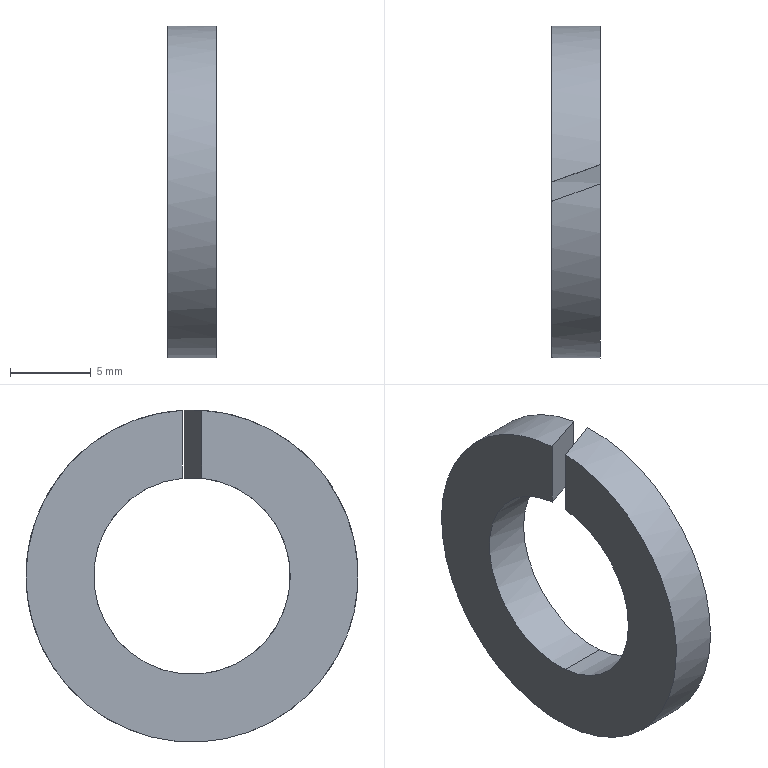Part | STEP file | KS B 1324 - No. 2 - 12 | 1 solid | 8 faces | box 3 x 20.6 x 20.6 mm | volume 633.995 mm3 | cylinder 4 | plane 4 | commonest cylinder face diameters 12.2 x2 20.6 x2
STEP:
#1=CARTESIAN_POINT('',(0.,0.,0.));
#2=DIRECTION('',(0.,0.,1.));
#3=DIRECTION('',(1.,0.,0.));
#4=AXIS2_PLACEMENT_3D('',#1,#2,#3);
#5=CARTESIAN_POINT('',(3.,1.692,5.861));
#6=VERTEX_POINT('',#5);
#7=CARTESIAN_POINT('',(0.,0.6,6.07));
#8=VERTEX_POINT('',#7);
#9=CARTESIAN_POINT('',(3.,1.692,5.861));
#10=CARTESIAN_POINT('',(2.019,1.335,5.964));
#11=CARTESIAN_POINT('',(1.016,0.9699,6.034));
#12=CARTESIAN_POINT('',(0.,0.6,6.07));
#13=(BOUNDED_CURVE()B_SPLINE_CURVE(3,(#9,#10,#11,#12),.UNSPECIFIED.,.F.,.F.)B_SPLINE_CURVE_WITH_KNOTS((4,4),(4.431,4.614),.PIECEWISE_BEZIER_KNOTS.)CURVE()GEOMETRIC_REPRESENTATION_ITEM()RATIONAL_B_SPLINE_CURVE((1.,0.9972,0.9972,1.))REPRESENTATION_ITEM(''));
#14=CARTESIAN_POINT('',(0.,0.,0.));
#15=DIRECTION('',(1.,0.,0.));
#16=DIRECTION('',(0.,-0.0895,-0.996));
#17=AXIS2_PLACEMENT_3D('',#14,#15,#16);
#18=CYLINDRICAL_SURFACE('',#17,6.1);
#19=CARTESIAN_POINT('',(2.95,3.));
#20=CARTESIAN_POINT('',(2.953,2.956));
#21=CARTESIAN_POINT('',(2.958,2.866));
#22=CARTESIAN_POINT('',(2.967,2.733));
#23=CARTESIAN_POINT('',(2.975,2.598));
#24=CARTESIAN_POINT('',(2.983,2.464));
#25=CARTESIAN_POINT('',(2.992,2.329));
#26=CARTESIAN_POINT('',(3.,2.193));
#27=CARTESIAN_POINT('',(3.008,2.058));
#28=CARTESIAN_POINT('',(3.017,1.922));
#29=CARTESIAN_POINT('',(3.025,1.786));
#30=CARTESIAN_POINT('',(3.033,1.65));
#31=CARTESIAN_POINT('',(3.041,1.513));
#32=CARTESIAN_POINT('',(3.05,1.376));
#33=CARTESIAN_POINT('',(3.058,1.239));
#34=CARTESIAN_POINT('',(3.066,1.102));
#35=CARTESIAN_POINT('',(3.075,0.965));
#36=CARTESIAN_POINT('',(3.083,0.8275));
#37=CARTESIAN_POINT('',(3.091,0.6899));
#38=CARTESIAN_POINT('',(3.1,0.5521));
#39=CARTESIAN_POINT('',(3.108,0.4142));
#40=CARTESIAN_POINT('',(3.116,0.2762));
#41=CARTESIAN_POINT('',(3.124,0.1382));
#42=CARTESIAN_POINT('',(3.13,0.04606));
#43=CARTESIAN_POINT('',(3.133,0.));
#44=B_SPLINE_CURVE_WITH_KNOTS('',3,(#19,#20,#21,#22,#23,#24,#25,#26,#27,#28,#29,#30,#31,#32,#33,#34,#35,#36,#37,#38,#39,#40,#41,#42,#43),.UNSPECIFIED.,.F.,.F.,(4,1,1,1,1,1,1,1,1,1,1,1,1,1,1,1,1,1,1,1,1,1,4),(4.431,4.44,4.448,4.456,4.465,4.473,4.481,4.489,4.498,4.506,4.514,4.523,4.531,4.539,4.547,4.556,4.564,4.572,4.581,4.589,4.597,4.606,4.614),.QUASI_UNIFORM_KNOTS.);
#45=(GEOMETRIC_REPRESENTATION_CONTEXT(2)PARAMETRIC_REPRESENTATION_CONTEXT()REPRESENTATION_CONTEXT('',''));
#46=DEFINITIONAL_REPRESENTATION('',(#44),#45);
#47=PCURVE('',#18,#46);
#48=CARTESIAN_POINT('',(0.,0.6,0.));
#49=DIRECTION('',(-0.342,0.9397,0.));
#50=DIRECTION('',(0.,0.,1.));
#51=AXIS2_PLACEMENT_3D('',#48,#49,#50);
#52=PLANE('',#51);
#53=CARTESIAN_POINT('',(5.861,3.193));
#54=CARTESIAN_POINT('',(5.964,2.149));
#55=CARTESIAN_POINT('',(6.034,1.081));
#56=CARTESIAN_POINT('',(6.07,0.));
#57=(BOUNDED_CURVE()B_SPLINE_CURVE(3,(#53,#54,#55,#56),.UNSPECIFIED.,.F.,.F.)B_SPLINE_CURVE_WITH_KNOTS((4,4),(4.431,4.614),.PIECEWISE_BEZIER_KNOTS.)CURVE()GEOMETRIC_REPRESENTATION_ITEM()RATIONAL_B_SPLINE_CURVE((1.,0.9972,0.9972,1.))REPRESENTATION_ITEM(''));
#58=(GEOMETRIC_REPRESENTATION_CONTEXT(2)PARAMETRIC_REPRESENTATION_CONTEXT()REPRESENTATION_CONTEXT('',''));
#59=DEFINITIONAL_REPRESENTATION('',(#57),#58);
#60=PCURVE('',#52,#59);
#61=SURFACE_CURVE('',#13,(#47,#60),.PCURVE_S1.);
#62=EDGE_CURVE('',#6,#8,#61,.T.);
#63=ORIENTED_EDGE('',*,*,#62,.F.);
#64=CARTESIAN_POINT('',(3.,-0.546,-6.076));
#65=VERTEX_POINT('',#64);
#66=CARTESIAN_POINT('',(3.,0.,0.));
#67=DIRECTION('',(-1.,0.,0.));
#68=DIRECTION('',(0.,-1.,0.));
#69=AXIS2_PLACEMENT_3D('',#66,#67,#68);
#70=CIRCLE('',#69,6.1);
#71=CARTESIAN_POINT('',(4.802,3.));
#72=DIRECTION('',(-1.,0.));
#73=VECTOR('',#72,1.);
#74=LINE('',#71,#73);
#75=(GEOMETRIC_REPRESENTATION_CONTEXT(2)PARAMETRIC_REPRESENTATION_CONTEXT()REPRESENTATION_CONTEXT('',''));
#76=DEFINITIONAL_REPRESENTATION('',(#74),#75);
#77=PCURVE('',#18,#76);
#78=CARTESIAN_POINT('',(3.,0.,0.));
#79=DIRECTION('',(-1.,0.,0.));
#80=DIRECTION('',(0.,0.,1.));
#81=AXIS2_PLACEMENT_3D('',#78,#79,#80);
#82=PLANE('',#81);
#83=CARTESIAN_POINT('',(0.,0.));
#84=DIRECTION('',(0.,-1.));
#85=AXIS2_PLACEMENT_2D('',#83,#84);
#86=CIRCLE('',#85,6.1);
#87=(GEOMETRIC_REPRESENTATION_CONTEXT(2)PARAMETRIC_REPRESENTATION_CONTEXT()REPRESENTATION_CONTEXT('',''));
#88=DEFINITIONAL_REPRESENTATION('',(#86),#87);
#89=PCURVE('',#82,#88);
#90=SURFACE_CURVE('',#70,(#77,#89),.PCURVE_S1.);
#91=EDGE_CURVE('',#6,#65,#90,.T.);
#92=ORIENTED_EDGE('',*,*,#91,.T.);
#93=CARTESIAN_POINT('',(0.,-0.546,-6.076));
#94=VERTEX_POINT('',#93);
#95=CARTESIAN_POINT('',(0.,-0.546,-6.076));
#96=DIRECTION('',(1.,0.,0.));
#97=VECTOR('',#96,1.);
#98=LINE('',#95,#97);
#99=CARTESIAN_POINT('',(0.,0.));
#100=DIRECTION('',(0.,1.));
#101=VECTOR('',#100,1.);
#102=LINE('',#99,#101);
#103=(GEOMETRIC_REPRESENTATION_CONTEXT(2)PARAMETRIC_REPRESENTATION_CONTEXT()REPRESENTATION_CONTEXT('',''));
#104=DEFINITIONAL_REPRESENTATION('',(#102),#103);
#105=PCURVE('',#18,#104);
#106=CARTESIAN_POINT('',(0.,0.,0.));
#107=DIRECTION('',(1.,0.,0.));
#108=DIRECTION('',(0.,-0.0895,-0.996));
#109=AXIS2_PLACEMENT_3D('',#106,#107,#108);
#110=CYLINDRICAL_SURFACE('',#109,6.1);
#111=CARTESIAN_POINT('',(6.283,0.));
#112=DIRECTION('',(0.,1.));
#113=VECTOR('',#112,1.);
#114=LINE('',#111,#113);
#115=(GEOMETRIC_REPRESENTATION_CONTEXT(2)PARAMETRIC_REPRESENTATION_CONTEXT()REPRESENTATION_CONTEXT('',''));
#116=DEFINITIONAL_REPRESENTATION('',(#114),#115);
#117=PCURVE('',#110,#116);
#118=SURFACE_CURVE('',#98,(#105,#117),.PCURVE_S1.);
#119=EDGE_CURVE('',#94,#65,#118,.T.);
#120=ORIENTED_EDGE('',*,*,#119,.F.);
#121=CARTESIAN_POINT('',(0.,0.,0.));
#122=DIRECTION('',(1.,0.,0.));
#123=DIRECTION('',(0.,-1.,0.));
#124=AXIS2_PLACEMENT_3D('',#121,#122,#123);
#125=CIRCLE('',#124,6.1);
#126=CARTESIAN_POINT('',(-1.481,0.));
#127=DIRECTION('',(1.,0.));
#128=VECTOR('',#127,1.);
#129=LINE('',#126,#128);
#130=(GEOMETRIC_REPRESENTATION_CONTEXT(2)PARAMETRIC_REPRESENTATION_CONTEXT()REPRESENTATION_CONTEXT('',''));
#131=DEFINITIONAL_REPRESENTATION('',(#129),#130);
#132=PCURVE('',#18,#131);
#133=CARTESIAN_POINT('',(0.,0.,0.));
#134=DIRECTION('',(-1.,0.,0.));
#135=DIRECTION('',(0.,0.,1.));
#136=AXIS2_PLACEMENT_3D('',#133,#134,#135);
#137=PLANE('',#136);
#138=CARTESIAN_POINT('',(0.,-6.1));
#139=CARTESIAN_POINT('',(-10.566,-6.1));
#140=CARTESIAN_POINT('',(-5.283,3.05));
#141=CARTESIAN_POINT('',(0.,12.2));
#142=CARTESIAN_POINT('',(5.283,3.05));
#143=CARTESIAN_POINT('',(10.566,-6.1));
#144=CARTESIAN_POINT('',(0.,-6.1));
#145=(BOUNDED_CURVE()B_SPLINE_CURVE(2,(#138,#139,#140,#141,#142,#143,#144),.UNSPECIFIED.,.T.,.F.)B_SPLINE_CURVE_WITH_KNOTS((1,2,2,2,2,1),(-2.094,0.,2.094,4.189,6.283,8.378),.UNSPECIFIED.)CURVE()GEOMETRIC_REPRESENTATION_ITEM()RATIONAL_B_SPLINE_CURVE((1.,0.5,1.,0.5,1.,0.5,1.))REPRESENTATION_ITEM(''));
#146=(GEOMETRIC_REPRESENTATION_CONTEXT(2)PARAMETRIC_REPRESENTATION_CONTEXT()REPRESENTATION_CONTEXT('',''));
#147=DEFINITIONAL_REPRESENTATION('',(#145),#146);
#148=PCURVE('',#137,#147);
#149=SURFACE_CURVE('',#125,(#132,#148),.PCURVE_S1.);
#150=EDGE_CURVE('',#94,#8,#149,.T.);
#151=ORIENTED_EDGE('',*,*,#150,.T.);
#152=EDGE_LOOP('',(#63,#92,#120,#151));
#153=FACE_BOUND('',#152,.F.);
#154=ADVANCED_FACE('',(#153),#18,.F.);
#155=CARTESIAN_POINT('',(0.,-0.546,-10.286));
#156=VERTEX_POINT('',#155);
#157=CARTESIAN_POINT('',(0.,-0.6,10.283));
#158=VERTEX_POINT('',#157);
#159=CARTESIAN_POINT('',(0.,0.,0.));
#160=DIRECTION('',(-1.,0.,0.));
#161=DIRECTION('',(0.,-1.,0.));
#162=AXIS2_PLACEMENT_3D('',#159,#160,#161);
#163=CIRCLE('',#162,10.3);
#164=CARTESIAN_POINT('',(0.,0.,0.));
#165=DIRECTION('',(1.,0.,0.));
#166=DIRECTION('',(0.,-0.05301,-0.9986));
#167=AXIS2_PLACEMENT_3D('',#164,#165,#166);
#168=CYLINDRICAL_SURFACE('',#167,10.3);
#169=CARTESIAN_POINT('',(11.049,0.));
#170=DIRECTION('',(-1.,0.));
#171=VECTOR('',#170,1.);
#172=LINE('',#169,#171);
#173=(GEOMETRIC_REPRESENTATION_CONTEXT(2)PARAMETRIC_REPRESENTATION_CONTEXT()REPRESENTATION_CONTEXT('',''));
#174=DEFINITIONAL_REPRESENTATION('',(#172),#173);
#175=PCURVE('',#168,#174);
#176=CARTESIAN_POINT('',(0.,0.));
#177=DIRECTION('',(0.,-1.));
#178=AXIS2_PLACEMENT_2D('',#176,#177);
#179=CIRCLE('',#178,10.3);
#180=(GEOMETRIC_REPRESENTATION_CONTEXT(2)PARAMETRIC_REPRESENTATION_CONTEXT()REPRESENTATION_CONTEXT('',''));
#181=DEFINITIONAL_REPRESENTATION('',(#179),#180);
#182=PCURVE('',#137,#181);
#183=SURFACE_CURVE('',#163,(#175,#182),.PCURVE_S1.);
#184=EDGE_CURVE('',#156,#158,#183,.T.);
#185=ORIENTED_EDGE('',*,*,#184,.F.);
#186=CARTESIAN_POINT('',(3.,-0.546,-10.286));
#187=VERTEX_POINT('',#186);
#188=CARTESIAN_POINT('',(0.,-0.546,-10.286));
#189=DIRECTION('',(1.,0.,0.));
#190=VECTOR('',#189,1.);
#191=LINE('',#188,#190);
#192=CARTESIAN_POINT('',(6.283,0.));
#193=DIRECTION('',(0.,1.));
#194=VECTOR('',#193,1.);
#195=LINE('',#192,#194);
#196=(GEOMETRIC_REPRESENTATION_CONTEXT(2)PARAMETRIC_REPRESENTATION_CONTEXT()REPRESENTATION_CONTEXT('',''));
#197=DEFINITIONAL_REPRESENTATION('',(#195),#196);
#198=PCURVE('',#168,#197);
#199=CARTESIAN_POINT('',(0.,0.,0.));
#200=DIRECTION('',(1.,0.,0.));
#201=DIRECTION('',(0.,-0.05301,-0.9986));
#202=AXIS2_PLACEMENT_3D('',#199,#200,#201);
#203=CYLINDRICAL_SURFACE('',#202,10.3);
#204=CARTESIAN_POINT('',(0.,0.));
#205=DIRECTION('',(0.,1.));
#206=VECTOR('',#205,1.);
#207=LINE('',#204,#206);
#208=(GEOMETRIC_REPRESENTATION_CONTEXT(2)PARAMETRIC_REPRESENTATION_CONTEXT()REPRESENTATION_CONTEXT('',''));
#209=DEFINITIONAL_REPRESENTATION('',(#207),#208);
#210=PCURVE('',#203,#209);
#211=SURFACE_CURVE('',#191,(#198,#210),.PCURVE_S1.);
#212=EDGE_CURVE('',#156,#187,#211,.T.);
#213=ORIENTED_EDGE('',*,*,#212,.T.);
#214=CARTESIAN_POINT('',(3.,0.4919,10.288));
#215=VERTEX_POINT('',#214);
#216=CARTESIAN_POINT('',(3.,0.,0.));
#217=DIRECTION('',(-1.,0.,0.));
#218=DIRECTION('',(0.,-1.,0.));
#219=AXIS2_PLACEMENT_3D('',#216,#217,#218);
#220=CIRCLE('',#219,10.3);
#221=CARTESIAN_POINT('',(11.049,3.));
#222=DIRECTION('',(-1.,0.));
#223=VECTOR('',#222,1.);
#224=LINE('',#221,#223);
#225=(GEOMETRIC_REPRESENTATION_CONTEXT(2)PARAMETRIC_REPRESENTATION_CONTEXT()REPRESENTATION_CONTEXT('',''));
#226=DEFINITIONAL_REPRESENTATION('',(#224),#225);
#227=PCURVE('',#168,#226);
#228=CARTESIAN_POINT('',(0.,0.));
#229=DIRECTION('',(0.,-1.));
#230=AXIS2_PLACEMENT_2D('',#228,#229);
#231=CIRCLE('',#230,10.3);
#232=(GEOMETRIC_REPRESENTATION_CONTEXT(2)PARAMETRIC_REPRESENTATION_CONTEXT()REPRESENTATION_CONTEXT('',''));
#233=DEFINITIONAL_REPRESENTATION('',(#231),#232);
#234=PCURVE('',#82,#233);
#235=SURFACE_CURVE('',#220,(#227,#234),.PCURVE_S1.);
#236=EDGE_CURVE('',#187,#215,#235,.T.);
#237=ORIENTED_EDGE('',*,*,#236,.T.);
#238=CARTESIAN_POINT('',(3.,0.4919,10.288));
#239=CARTESIAN_POINT('',(2.,0.128,10.306));
#240=CARTESIAN_POINT('',(0.9993,-0.2363,10.304));
#241=CARTESIAN_POINT('',(0.,-0.6,10.283));
#242=(BOUNDED_CURVE()B_SPLINE_CURVE(3,(#238,#239,#240,#241),.UNSPECIFIED.,.F.,.F.)B_SPLINE_CURVE_WITH_KNOTS((4,4),(4.665,4.771),.PIECEWISE_BEZIER_KNOTS.)CURVE()GEOMETRIC_REPRESENTATION_ITEM()RATIONAL_B_SPLINE_CURVE((1.,0.9991,0.9991,1.))REPRESENTATION_ITEM(''));
#243=CARTESIAN_POINT('',(3.147,3.));
#244=CARTESIAN_POINT('',(3.148,2.955));
#245=CARTESIAN_POINT('',(3.152,2.864));
#246=CARTESIAN_POINT('',(3.156,2.727));
#247=CARTESIAN_POINT('',(3.161,2.591));
#248=CARTESIAN_POINT('',(3.166,2.455));
#249=CARTESIAN_POINT('',(3.171,2.318));
#250=CARTESIAN_POINT('',(3.176,2.182));
#251=CARTESIAN_POINT('',(3.181,2.046));
#252=CARTESIAN_POINT('',(3.185,1.909));
#253=CARTESIAN_POINT('',(3.19,1.773));
#254=CARTESIAN_POINT('',(3.195,1.636));
#255=CARTESIAN_POINT('',(3.2,1.5));
#256=CARTESIAN_POINT('',(3.205,1.363));
#257=CARTESIAN_POINT('',(3.21,1.227));
#258=CARTESIAN_POINT('',(3.214,1.09));
#259=CARTESIAN_POINT('',(3.219,0.954));
#260=CARTESIAN_POINT('',(3.224,0.8176));
#261=CARTESIAN_POINT('',(3.229,0.6813));
#262=CARTESIAN_POINT('',(3.234,0.5449));
#263=CARTESIAN_POINT('',(3.238,0.4086));
#264=CARTESIAN_POINT('',(3.243,0.2724));
#265=CARTESIAN_POINT('',(3.248,0.1362));
#266=CARTESIAN_POINT('',(3.251,0.04538));
#267=CARTESIAN_POINT('',(3.253,0.));
#268=B_SPLINE_CURVE_WITH_KNOTS('',3,(#243,#244,#245,#246,#247,#248,#249,#250,#251,#252,#253,#254,#255,#256,#257,#258,#259,#260,#261,#262,#263,#264,#265,#266,#267),.UNSPECIFIED.,.F.,.F.,(4,1,1,1,1,1,1,1,1,1,1,1,1,1,1,1,1,1,1,1,1,1,4),(4.665,4.669,4.674,4.679,4.684,4.689,4.694,4.698,4.703,4.708,4.713,4.718,4.722,4.727,4.732,4.737,4.742,4.747,4.751,4.756,4.761,4.766,4.771),.QUASI_UNIFORM_KNOTS.);
#269=(GEOMETRIC_REPRESENTATION_CONTEXT(2)PARAMETRIC_REPRESENTATION_CONTEXT()REPRESENTATION_CONTEXT('',''));
#270=DEFINITIONAL_REPRESENTATION('',(#268),#269);
#271=PCURVE('',#168,#270);
#272=CARTESIAN_POINT('',(3.,0.4919,0.));
#273=DIRECTION('',(0.342,-0.9397,0.));
#274=DIRECTION('',(0.,0.,-1.));
#275=AXIS2_PLACEMENT_3D('',#272,#273,#274);
#276=PLANE('',#275);
#277=CARTESIAN_POINT('',(-10.288,0.));
#278=CARTESIAN_POINT('',(-10.306,-1.064));
#279=CARTESIAN_POINT('',(-10.304,-2.129));
#280=CARTESIAN_POINT('',(-10.283,-3.193));
#281=(BOUNDED_CURVE()B_SPLINE_CURVE(3,(#277,#278,#279,#280),.UNSPECIFIED.,.F.,.F.)B_SPLINE_CURVE_WITH_KNOTS((4,4),(4.665,4.771),.PIECEWISE_BEZIER_KNOTS.)CURVE()GEOMETRIC_REPRESENTATION_ITEM()RATIONAL_B_SPLINE_CURVE((1.,0.9991,0.9991,1.))REPRESENTATION_ITEM(''));
#282=(GEOMETRIC_REPRESENTATION_CONTEXT(2)PARAMETRIC_REPRESENTATION_CONTEXT()REPRESENTATION_CONTEXT('',''));
#283=DEFINITIONAL_REPRESENTATION('',(#281),#282);
#284=PCURVE('',#276,#283);
#285=SURFACE_CURVE('',#242,(#271,#284),.PCURVE_S1.);
#286=EDGE_CURVE('',#215,#158,#285,.T.);
#287=ORIENTED_EDGE('',*,*,#286,.T.);
#288=EDGE_LOOP('',(#185,#213,#237,#287));
#289=FACE_BOUND('',#288,.T.);
#290=ADVANCED_FACE('',(#289),#168,.T.);
#291=CARTESIAN_POINT('',(0.,-0.6,6.07));
#292=VERTEX_POINT('',#291);
#293=CARTESIAN_POINT('',(0.,-0.6,0.));
#294=DIRECTION('',(0.,0.,-1.));
#295=VECTOR('',#294,1.);
#296=LINE('',#293,#295);
#297=CARTESIAN_POINT('',(0.,-0.6));
#298=DIRECTION('',(-1.,0.));
#299=VECTOR('',#298,1.);
#300=LINE('',#297,#299);
#301=(GEOMETRIC_REPRESENTATION_CONTEXT(2)PARAMETRIC_REPRESENTATION_CONTEXT()REPRESENTATION_CONTEXT('',''));
#302=DEFINITIONAL_REPRESENTATION('',(#300),#301);
#303=PCURVE('',#137,#302);
#304=CARTESIAN_POINT('',(0.,-3.193));
#305=DIRECTION('',(1.,0.));
#306=VECTOR('',#305,1.);
#307=LINE('',#304,#306);
#308=(GEOMETRIC_REPRESENTATION_CONTEXT(2)PARAMETRIC_REPRESENTATION_CONTEXT()REPRESENTATION_CONTEXT('',''));
#309=DEFINITIONAL_REPRESENTATION('',(#307),#308);
#310=PCURVE('',#276,#309);
#311=SURFACE_CURVE('',#296,(#303,#310),.PCURVE_S1.);
#312=EDGE_CURVE('',#158,#292,#311,.T.);
#313=ORIENTED_EDGE('',*,*,#312,.T.);
#314=CARTESIAN_POINT('',(0.,0.,0.));
#315=DIRECTION('',(1.,0.,0.));
#316=DIRECTION('',(0.,-1.,0.));
#317=AXIS2_PLACEMENT_3D('',#314,#315,#316);
#318=CIRCLE('',#317,6.1);
#319=CARTESIAN_POINT('',(0.,-6.1));
#320=CARTESIAN_POINT('',(-10.566,-6.1));
#321=CARTESIAN_POINT('',(-5.283,3.05));
#322=CARTESIAN_POINT('',(0.,12.2));
#323=CARTESIAN_POINT('',(5.283,3.05));
#324=CARTESIAN_POINT('',(10.566,-6.1));
#325=CARTESIAN_POINT('',(0.,-6.1));
#326=(BOUNDED_CURVE()B_SPLINE_CURVE(2,(#319,#320,#321,#322,#323,#324,#325),.UNSPECIFIED.,.T.,.F.)B_SPLINE_CURVE_WITH_KNOTS((1,2,2,2,2,1),(-2.094,0.,2.094,4.189,6.283,8.378),.UNSPECIFIED.)CURVE()GEOMETRIC_REPRESENTATION_ITEM()RATIONAL_B_SPLINE_CURVE((1.,0.5,1.,0.5,1.,0.5,1.))REPRESENTATION_ITEM(''));
#327=(GEOMETRIC_REPRESENTATION_CONTEXT(2)PARAMETRIC_REPRESENTATION_CONTEXT()REPRESENTATION_CONTEXT('',''));
#328=DEFINITIONAL_REPRESENTATION('',(#326),#327);
#329=PCURVE('',#137,#328);
#330=CARTESIAN_POINT('',(-1.481,0.));
#331=DIRECTION('',(1.,0.));
#332=VECTOR('',#331,1.);
#333=LINE('',#330,#332);
#334=(GEOMETRIC_REPRESENTATION_CONTEXT(2)PARAMETRIC_REPRESENTATION_CONTEXT()REPRESENTATION_CONTEXT('',''));
#335=DEFINITIONAL_REPRESENTATION('',(#333),#334);
#336=PCURVE('',#110,#335);
#337=SURFACE_CURVE('',#318,(#329,#336),.PCURVE_S1.);
#338=EDGE_CURVE('',#292,#94,#337,.T.);
#339=ORIENTED_EDGE('',*,*,#338,.T.);
#340=ORIENTED_EDGE('',*,*,#150,.T.);
#341=CARTESIAN_POINT('',(0.,0.6,10.283));
#342=VERTEX_POINT('',#341);
#343=CARTESIAN_POINT('',(0.,0.6,0.));
#344=DIRECTION('',(0.,0.,1.));
#345=VECTOR('',#344,1.);
#346=LINE('',#343,#345);
#347=CARTESIAN_POINT('',(0.,0.6));
#348=DIRECTION('',(1.,0.));
#349=VECTOR('',#348,1.);
#350=LINE('',#347,#349);
#351=(GEOMETRIC_REPRESENTATION_CONTEXT(2)PARAMETRIC_REPRESENTATION_CONTEXT()REPRESENTATION_CONTEXT('',''));
#352=DEFINITIONAL_REPRESENTATION('',(#350),#351);
#353=PCURVE('',#137,#352);
#354=CARTESIAN_POINT('',(0.,0.));
#355=DIRECTION('',(1.,0.));
#356=VECTOR('',#355,1.);
#357=LINE('',#354,#356);
#358=(GEOMETRIC_REPRESENTATION_CONTEXT(2)PARAMETRIC_REPRESENTATION_CONTEXT()REPRESENTATION_CONTEXT('',''));
#359=DEFINITIONAL_REPRESENTATION('',(#357),#358);
#360=PCURVE('',#52,#359);
#361=SURFACE_CURVE('',#346,(#353,#360),.PCURVE_S1.);
#362=EDGE_CURVE('',#8,#342,#361,.T.);
#363=ORIENTED_EDGE('',*,*,#362,.T.);
#364=CARTESIAN_POINT('',(0.,0.,0.));
#365=DIRECTION('',(-1.,0.,0.));
#366=DIRECTION('',(0.,-1.,0.));
#367=AXIS2_PLACEMENT_3D('',#364,#365,#366);
#368=CIRCLE('',#367,10.3);
#369=CARTESIAN_POINT('',(0.,0.));
#370=DIRECTION('',(0.,-1.));
#371=AXIS2_PLACEMENT_2D('',#369,#370);
#372=CIRCLE('',#371,10.3);
#373=(GEOMETRIC_REPRESENTATION_CONTEXT(2)PARAMETRIC_REPRESENTATION_CONTEXT()REPRESENTATION_CONTEXT('',''));
#374=DEFINITIONAL_REPRESENTATION('',(#372),#373);
#375=PCURVE('',#137,#374);
#376=CARTESIAN_POINT('',(4.765,0.));
#377=DIRECTION('',(-1.,0.));
#378=VECTOR('',#377,1.);
#379=LINE('',#376,#378);
#380=(GEOMETRIC_REPRESENTATION_CONTEXT(2)PARAMETRIC_REPRESENTATION_CONTEXT()REPRESENTATION_CONTEXT('',''));
#381=DEFINITIONAL_REPRESENTATION('',(#379),#380);
#382=PCURVE('',#203,#381);
#383=SURFACE_CURVE('',#368,(#375,#382),.PCURVE_S1.);
#384=EDGE_CURVE('',#342,#156,#383,.T.);
#385=ORIENTED_EDGE('',*,*,#384,.T.);
#386=ORIENTED_EDGE('',*,*,#184,.T.);
#387=EDGE_LOOP('',(#313,#339,#340,#363,#385,#386));
#388=FACE_BOUND('',#387,.T.);
#389=ADVANCED_FACE('',(#388),#137,.T.);
#390=ORIENTED_EDGE('',*,*,#212,.F.);
#391=ORIENTED_EDGE('',*,*,#384,.F.);
#392=CARTESIAN_POINT('',(3.,1.692,10.16));
#393=VERTEX_POINT('',#392);
#394=CARTESIAN_POINT('',(0.,0.6,10.283));
#395=CARTESIAN_POINT('',(1.006,0.966,10.261));
#396=CARTESIAN_POINT('',(2.006,1.33,10.22));
#397=CARTESIAN_POINT('',(3.,1.692,10.16));
#398=(BOUNDED_CURVE()B_SPLINE_CURVE(3,(#394,#395,#396,#397),.UNSPECIFIED.,.F.,.F.)B_SPLINE_CURVE_WITH_KNOTS((4,4),(1.629,1.736),.PIECEWISE_BEZIER_KNOTS.)CURVE()GEOMETRIC_REPRESENTATION_ITEM()RATIONAL_B_SPLINE_CURVE((1.,0.9991,0.9991,1.))REPRESENTATION_ITEM(''));
#399=CARTESIAN_POINT('',(3.136,0.));
#400=CARTESIAN_POINT('',(3.135,0.04566));
#401=CARTESIAN_POINT('',(3.131,0.137));
#402=CARTESIAN_POINT('',(3.127,0.2739));
#403=CARTESIAN_POINT('',(3.122,0.4108));
#404=CARTESIAN_POINT('',(3.117,0.5477));
#405=CARTESIAN_POINT('',(3.112,0.6846));
#406=CARTESIAN_POINT('',(3.107,0.8214));
#407=CARTESIAN_POINT('',(3.102,0.9581));
#408=CARTESIAN_POINT('',(3.098,1.095));
#409=CARTESIAN_POINT('',(3.093,1.231));
#410=CARTESIAN_POINT('',(3.088,1.368));
#411=CARTESIAN_POINT('',(3.083,1.505));
#412=CARTESIAN_POINT('',(3.078,1.641));
#413=CARTESIAN_POINT('',(3.073,1.777));
#414=CARTESIAN_POINT('',(3.068,1.914));
#415=CARTESIAN_POINT('',(3.064,2.05));
#416=CARTESIAN_POINT('',(3.059,2.186));
#417=CARTESIAN_POINT('',(3.054,2.322));
#418=CARTESIAN_POINT('',(3.049,2.458));
#419=CARTESIAN_POINT('',(3.044,2.593));
#420=CARTESIAN_POINT('',(3.039,2.729));
#421=CARTESIAN_POINT('',(3.034,2.865));
#422=CARTESIAN_POINT('',(3.031,2.955));
#423=CARTESIAN_POINT('',(3.03,3.));
#424=B_SPLINE_CURVE_WITH_KNOTS('',3,(#399,#400,#401,#402,#403,#404,#405,#406,#407,#408,#409,#410,#411,#412,#413,#414,#415,#416,#417,#418,#419,#420,#421,#422,#423),.UNSPECIFIED.,.F.,.F.,(4,1,1,1,1,1,1,1,1,1,1,1,1,1,1,1,1,1,1,1,1,1,4),(1.629,1.634,1.639,1.644,1.648,1.653,1.658,1.663,1.668,1.673,1.678,1.682,1.687,1.692,1.697,1.702,1.707,1.712,1.716,1.721,1.726,1.731,1.736),.QUASI_UNIFORM_KNOTS.);
#425=(GEOMETRIC_REPRESENTATION_CONTEXT(2)PARAMETRIC_REPRESENTATION_CONTEXT()REPRESENTATION_CONTEXT('',''));
#426=DEFINITIONAL_REPRESENTATION('',(#424),#425);
#427=PCURVE('',#203,#426);
#428=CARTESIAN_POINT('',(10.283,0.));
#429=CARTESIAN_POINT('',(10.261,1.07));
#430=CARTESIAN_POINT('',(10.22,2.135));
#431=CARTESIAN_POINT('',(10.16,3.193));
#432=(BOUNDED_CURVE()B_SPLINE_CURVE(3,(#428,#429,#430,#431),.UNSPECIFIED.,.F.,.F.)B_SPLINE_CURVE_WITH_KNOTS((4,4),(1.629,1.736),.PIECEWISE_BEZIER_KNOTS.)CURVE()GEOMETRIC_REPRESENTATION_ITEM()RATIONAL_B_SPLINE_CURVE((1.,0.9991,0.9991,1.))REPRESENTATION_ITEM(''));
#433=(GEOMETRIC_REPRESENTATION_CONTEXT(2)PARAMETRIC_REPRESENTATION_CONTEXT()REPRESENTATION_CONTEXT('',''));
#434=DEFINITIONAL_REPRESENTATION('',(#432),#433);
#435=PCURVE('',#52,#434);
#436=SURFACE_CURVE('',#398,(#427,#435),.PCURVE_S1.);
#437=EDGE_CURVE('',#342,#393,#436,.T.);
#438=ORIENTED_EDGE('',*,*,#437,.T.);
#439=CARTESIAN_POINT('',(3.,0.,0.));
#440=DIRECTION('',(-1.,0.,0.));
#441=DIRECTION('',(0.,-1.,0.));
#442=AXIS2_PLACEMENT_3D('',#439,#440,#441);
#443=CIRCLE('',#442,10.3);
#444=CARTESIAN_POINT('',(4.765,3.));
#445=DIRECTION('',(-1.,0.));
#446=VECTOR('',#445,1.);
#447=LINE('',#444,#446);
#448=(GEOMETRIC_REPRESENTATION_CONTEXT(2)PARAMETRIC_REPRESENTATION_CONTEXT()REPRESENTATION_CONTEXT('',''));
#449=DEFINITIONAL_REPRESENTATION('',(#447),#448);
#450=PCURVE('',#203,#449);
#451=CARTESIAN_POINT('',(0.,0.));
#452=DIRECTION('',(0.,-1.));
#453=AXIS2_PLACEMENT_2D('',#451,#452);
#454=CIRCLE('',#453,10.3);
#455=(GEOMETRIC_REPRESENTATION_CONTEXT(2)PARAMETRIC_REPRESENTATION_CONTEXT()REPRESENTATION_CONTEXT('',''));
#456=DEFINITIONAL_REPRESENTATION('',(#454),#455);
#457=PCURVE('',#82,#456);
#458=SURFACE_CURVE('',#443,(#450,#457),.PCURVE_S1.);
#459=EDGE_CURVE('',#393,#187,#458,.T.);
#460=ORIENTED_EDGE('',*,*,#459,.T.);
#461=EDGE_LOOP('',(#390,#391,#438,#460));
#462=FACE_BOUND('',#461,.T.);
#463=ADVANCED_FACE('',(#462),#203,.T.);
#464=CARTESIAN_POINT('',(3.,0.4919,6.08));
#465=VERTEX_POINT('',#464);
#466=CARTESIAN_POINT('',(3.,0.,0.));
#467=DIRECTION('',(-1.,0.,0.));
#468=DIRECTION('',(0.,-1.,0.));
#469=AXIS2_PLACEMENT_3D('',#466,#467,#468);
#470=CIRCLE('',#469,6.1);
#471=CARTESIAN_POINT('',(11.085,3.));
#472=DIRECTION('',(-1.,0.));
#473=VECTOR('',#472,1.);
#474=LINE('',#471,#473);
#475=(GEOMETRIC_REPRESENTATION_CONTEXT(2)PARAMETRIC_REPRESENTATION_CONTEXT()REPRESENTATION_CONTEXT('',''));
#476=DEFINITIONAL_REPRESENTATION('',(#474),#475);
#477=PCURVE('',#110,#476);
#478=CARTESIAN_POINT('',(0.,0.));
#479=DIRECTION('',(0.,-1.));
#480=AXIS2_PLACEMENT_2D('',#478,#479);
#481=CIRCLE('',#480,6.1);
#482=(GEOMETRIC_REPRESENTATION_CONTEXT(2)PARAMETRIC_REPRESENTATION_CONTEXT()REPRESENTATION_CONTEXT('',''));
#483=DEFINITIONAL_REPRESENTATION('',(#481),#482);
#484=PCURVE('',#82,#483);
#485=SURFACE_CURVE('',#470,(#477,#484),.PCURVE_S1.);
#486=EDGE_CURVE('',#65,#465,#485,.T.);
#487=ORIENTED_EDGE('',*,*,#486,.T.);
#488=CARTESIAN_POINT('',(0.,-0.6,6.07));
#489=CARTESIAN_POINT('',(0.9979,-0.2368,6.106));
#490=CARTESIAN_POINT('',(2.001,0.1281,6.11));
#491=CARTESIAN_POINT('',(3.,0.4919,6.08));
#492=(BOUNDED_CURVE()B_SPLINE_CURVE(3,(#488,#489,#490,#491),.UNSPECIFIED.,.F.,.F.)B_SPLINE_CURVE_WITH_KNOTS((4,4),(1.472,1.652),.PIECEWISE_BEZIER_KNOTS.)CURVE()GEOMETRIC_REPRESENTATION_ITEM()RATIONAL_B_SPLINE_CURVE((1.,0.9973,0.9973,1.))REPRESENTATION_ITEM(''));
#493=CARTESIAN_POINT('',(3.33,0.));
#494=CARTESIAN_POINT('',(3.327,0.04524));
#495=CARTESIAN_POINT('',(3.322,0.1358));
#496=CARTESIAN_POINT('',(3.313,0.2717));
#497=CARTESIAN_POINT('',(3.305,0.4078));
#498=CARTESIAN_POINT('',(3.297,0.5439));
#499=CARTESIAN_POINT('',(3.289,0.6802));
#500=CARTESIAN_POINT('',(3.281,0.8166));
#501=CARTESIAN_POINT('',(3.273,0.9531));
#502=CARTESIAN_POINT('',(3.265,1.09));
#503=CARTESIAN_POINT('',(3.256,1.226));
#504=CARTESIAN_POINT('',(3.248,1.363));
#505=CARTESIAN_POINT('',(3.24,1.499));
#506=CARTESIAN_POINT('',(3.232,1.636));
#507=CARTESIAN_POINT('',(3.224,1.773));
#508=CARTESIAN_POINT('',(3.216,1.909));
#509=CARTESIAN_POINT('',(3.208,2.046));
#510=CARTESIAN_POINT('',(3.199,2.182));
#511=CARTESIAN_POINT('',(3.191,2.319));
#512=CARTESIAN_POINT('',(3.183,2.455));
#513=CARTESIAN_POINT('',(3.175,2.592));
#514=CARTESIAN_POINT('',(3.167,2.728));
#515=CARTESIAN_POINT('',(3.159,2.864));
#516=CARTESIAN_POINT('',(3.153,2.955));
#517=CARTESIAN_POINT('',(3.15,3.));
#518=B_SPLINE_CURVE_WITH_KNOTS('',3,(#493,#494,#495,#496,#497,#498,#499,#500,#501,#502,#503,#504,#505,#506,#507,#508,#509,#510,#511,#512,#513,#514,#515,#516,#517),.UNSPECIFIED.,.F.,.F.,(4,1,1,1,1,1,1,1,1,1,1,1,1,1,1,1,1,1,1,1,1,1,4),(1.472,1.48,1.489,1.497,1.505,1.513,1.521,1.529,1.537,1.546,1.554,1.562,1.57,1.578,1.586,1.594,1.603,1.611,1.619,1.627,1.635,1.643,1.652),.QUASI_UNIFORM_KNOTS.);
#519=(GEOMETRIC_REPRESENTATION_CONTEXT(2)PARAMETRIC_REPRESENTATION_CONTEXT()REPRESENTATION_CONTEXT('',''));
#520=DEFINITIONAL_REPRESENTATION('',(#518),#519);
#521=PCURVE('',#110,#520);
#522=CARTESIAN_POINT('',(-6.07,-3.193));
#523=CARTESIAN_POINT('',(-6.106,-2.131));
#524=CARTESIAN_POINT('',(-6.11,-1.064));
#525=CARTESIAN_POINT('',(-6.08,0.));
#526=(BOUNDED_CURVE()B_SPLINE_CURVE(3,(#522,#523,#524,#525),.UNSPECIFIED.,.F.,.F.)B_SPLINE_CURVE_WITH_KNOTS((4,4),(1.472,1.652),.PIECEWISE_BEZIER_KNOTS.)CURVE()GEOMETRIC_REPRESENTATION_ITEM()RATIONAL_B_SPLINE_CURVE((1.,0.9973,0.9973,1.))REPRESENTATION_ITEM(''));
#527=(GEOMETRIC_REPRESENTATION_CONTEXT(2)PARAMETRIC_REPRESENTATION_CONTEXT()REPRESENTATION_CONTEXT('',''));
#528=DEFINITIONAL_REPRESENTATION('',(#526),#527);
#529=PCURVE('',#276,#528);
#530=SURFACE_CURVE('',#492,(#521,#529),.PCURVE_S1.);
#531=EDGE_CURVE('',#292,#465,#530,.T.);
#532=ORIENTED_EDGE('',*,*,#531,.F.);
#533=ORIENTED_EDGE('',*,*,#338,.T.);
#534=ORIENTED_EDGE('',*,*,#119,.T.);
#535=EDGE_LOOP('',(#487,#532,#533,#534));
#536=FACE_BOUND('',#535,.F.);
#537=ADVANCED_FACE('',(#536),#110,.F.);
#538=CARTESIAN_POINT('',(3.,0.4919,0.));
#539=DIRECTION('',(0.,0.,1.));
#540=VECTOR('',#539,1.);
#541=LINE('',#538,#540);
#542=CARTESIAN_POINT('',(0.,0.4919));
#543=DIRECTION('',(1.,0.));
#544=VECTOR('',#543,1.);
#545=LINE('',#542,#544);
#546=(GEOMETRIC_REPRESENTATION_CONTEXT(2)PARAMETRIC_REPRESENTATION_CONTEXT()REPRESENTATION_CONTEXT('',''));
#547=DEFINITIONAL_REPRESENTATION('',(#545),#546);
#548=PCURVE('',#82,#547);
#549=CARTESIAN_POINT('',(0.,0.));
#550=DIRECTION('',(-1.,0.));
#551=VECTOR('',#550,1.);
#552=LINE('',#549,#551);
#553=(GEOMETRIC_REPRESENTATION_CONTEXT(2)PARAMETRIC_REPRESENTATION_CONTEXT()REPRESENTATION_CONTEXT('',''));
#554=DEFINITIONAL_REPRESENTATION('',(#552),#553);
#555=PCURVE('',#276,#554);
#556=SURFACE_CURVE('',#541,(#548,#555),.PCURVE_S1.);
#557=EDGE_CURVE('',#465,#215,#556,.T.);
#558=ORIENTED_EDGE('',*,*,#557,.T.);
#559=ORIENTED_EDGE('',*,*,#236,.F.);
#560=ORIENTED_EDGE('',*,*,#459,.F.);
#561=CARTESIAN_POINT('',(3.,1.692,0.));
#562=DIRECTION('',(0.,0.,-1.));
#563=VECTOR('',#562,1.);
#564=LINE('',#561,#563);
#565=CARTESIAN_POINT('',(0.,1.692));
#566=DIRECTION('',(-1.,0.));
#567=VECTOR('',#566,1.);
#568=LINE('',#565,#567);
#569=(GEOMETRIC_REPRESENTATION_CONTEXT(2)PARAMETRIC_REPRESENTATION_CONTEXT()REPRESENTATION_CONTEXT('',''));
#570=DEFINITIONAL_REPRESENTATION('',(#568),#569);
#571=PCURVE('',#82,#570);
#572=CARTESIAN_POINT('',(0.,3.193));
#573=DIRECTION('',(-1.,0.));
#574=VECTOR('',#573,1.);
#575=LINE('',#572,#574);
#576=(GEOMETRIC_REPRESENTATION_CONTEXT(2)PARAMETRIC_REPRESENTATION_CONTEXT()REPRESENTATION_CONTEXT('',''));
#577=DEFINITIONAL_REPRESENTATION('',(#575),#576);
#578=PCURVE('',#52,#577);
#579=SURFACE_CURVE('',#564,(#571,#578),.PCURVE_S1.);
#580=EDGE_CURVE('',#393,#6,#579,.T.);
#581=ORIENTED_EDGE('',*,*,#580,.T.);
#582=ORIENTED_EDGE('',*,*,#91,.T.);
#583=ORIENTED_EDGE('',*,*,#486,.T.);
#584=EDGE_LOOP('',(#558,#559,#560,#581,#582,#583));
#585=FACE_BOUND('',#584,.T.);
#586=ADVANCED_FACE('',(#585),#82,.F.);
#587=ORIENTED_EDGE('',*,*,#531,.F.);
#588=ORIENTED_EDGE('',*,*,#312,.F.);
#589=ORIENTED_EDGE('',*,*,#286,.F.);
#590=ORIENTED_EDGE('',*,*,#557,.F.);
#591=EDGE_LOOP('',(#587,#588,#589,#590));
#592=FACE_BOUND('',#591,.T.);
#593=ADVANCED_FACE('',(#592),#276,.F.);
#594=ORIENTED_EDGE('',*,*,#62,.F.);
#595=ORIENTED_EDGE('',*,*,#580,.F.);
#596=ORIENTED_EDGE('',*,*,#437,.F.);
#597=ORIENTED_EDGE('',*,*,#362,.F.);
#598=EDGE_LOOP('',(#594,#595,#596,#597));
#599=FACE_BOUND('',#598,.T.);
#600=ADVANCED_FACE('',(#599),#52,.F.);
#601=CLOSED_SHELL('',(#154,#290,#389,#463,#537,#586,#593,#600));
#602=MANIFOLD_SOLID_BREP('',#601);
#603=(LENGTH_UNIT()NAMED_UNIT(*)SI_UNIT(.MILLI.,.METRE.));
#604=UNCERTAINTY_MEASURE_WITH_UNIT(LENGTH_MEASURE(0.0000001),#603,'','');
#605=(NAMED_UNIT(*)PLANE_ANGLE_UNIT()SI_UNIT($,.RADIAN.));
#606=(NAMED_UNIT(*)SI_UNIT($,.STERADIAN.)SOLID_ANGLE_UNIT());
#607=(GEOMETRIC_REPRESENTATION_CONTEXT(3)GLOBAL_UNCERTAINTY_ASSIGNED_CONTEXT((#604))GLOBAL_UNIT_ASSIGNED_CONTEXT((#603,#605,#606))REPRESENTATION_CONTEXT('',''));
#608=ADVANCED_BREP_SHAPE_REPRESENTATION('',(#4,#602),#607);